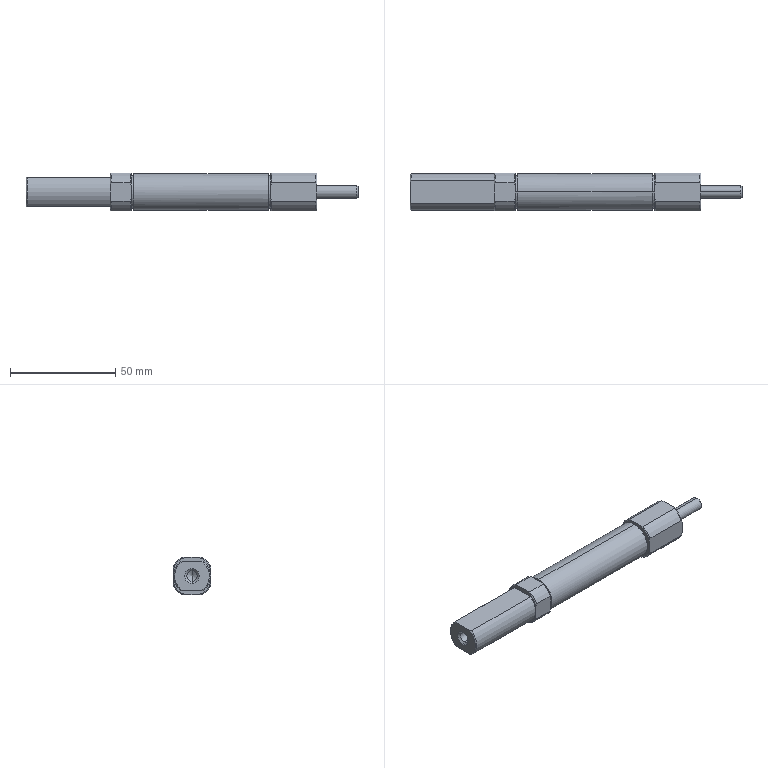Part | STEP file | 102000010554 | 2 solids | 76 faces | box 157.5 x 18 x 18 mm | volume 33195 mm3 | cone 28 | cylinder 28 | plane 20 | commonest cylinder face diameters 20 x8 4.2 x6 6 x4 15.5 x4 17.5 x4 5 x2